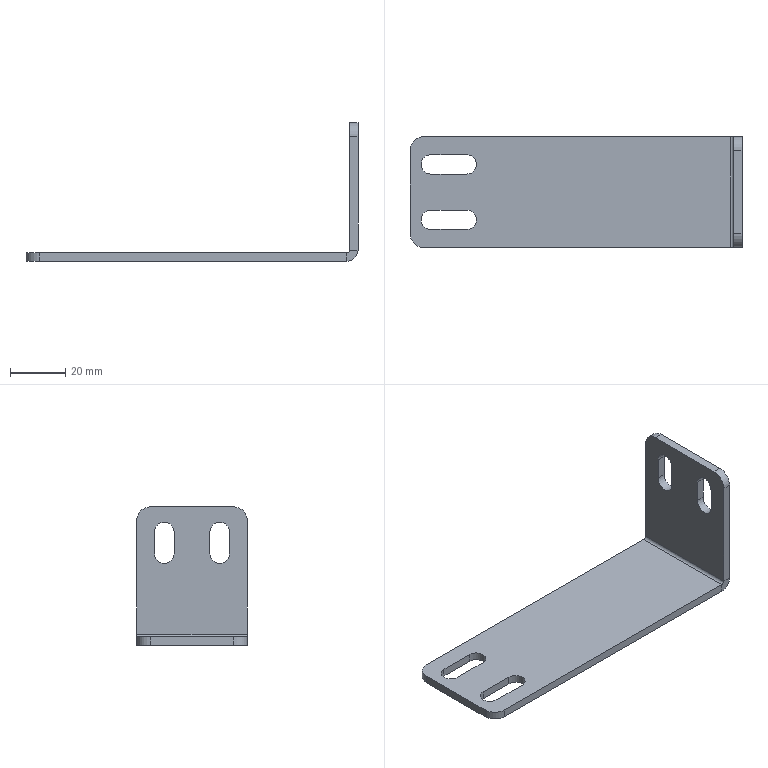Part | STEP file | PN_0007 L-type guardrail connecting plate 120X50_Default<As Machined> | 1 solid | 34 faces | box 120 x 40 x 50 mm | volume 18503 mm3 | plane 20 | cylinder 14 | commonest cylinder face diameters 7 x8 10 x4 2 x1 8 x1